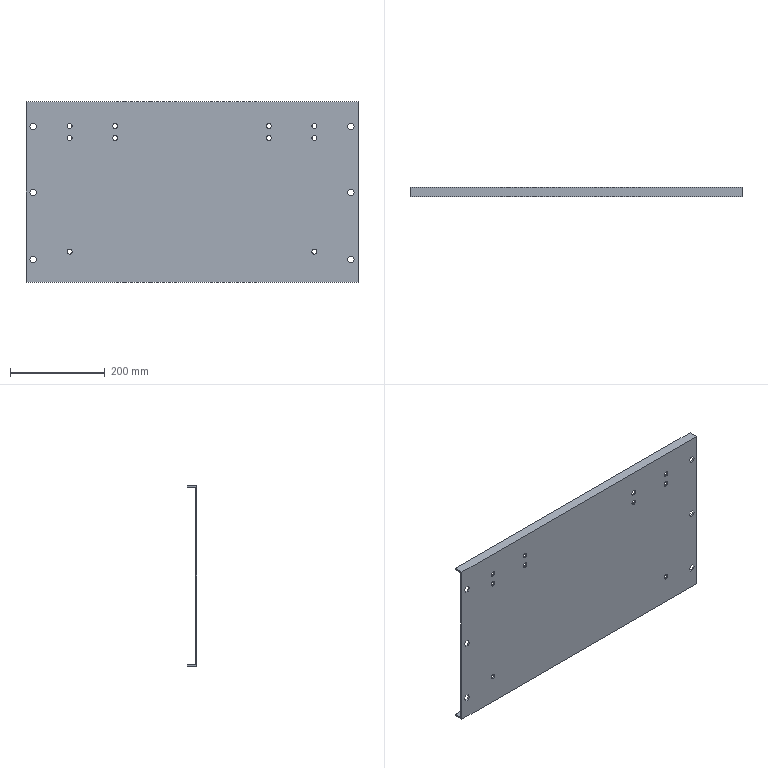Part | SolidWorks | features BaseBody 1 | 1 solid | 66 faces | box 700 x 20 x 380 mm | volume 864118 mm3 | plane 46 | cylinder 20 | commonest cylinder face diameters 10.6 x20